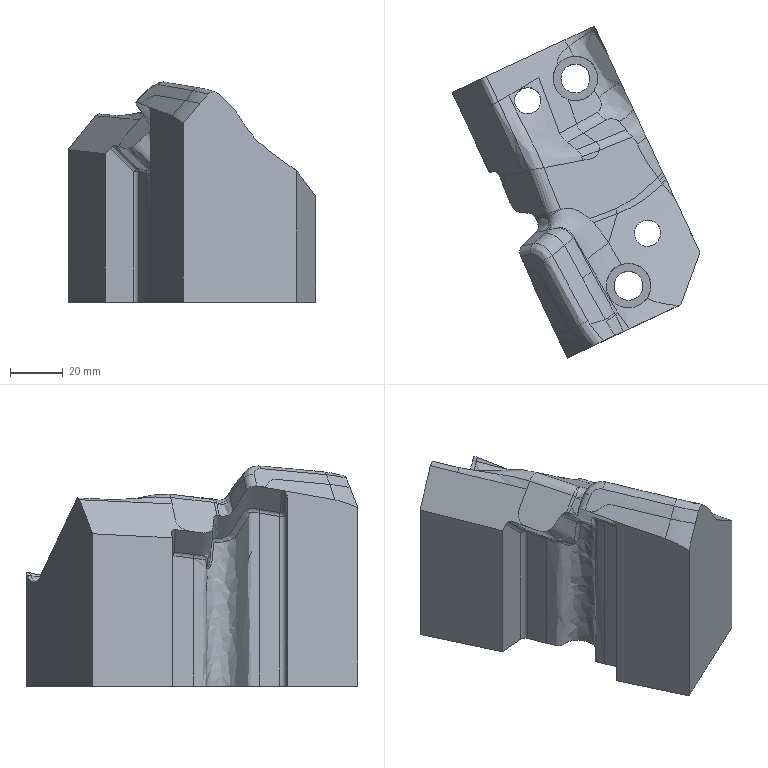Part | NX | features solid 2 | 1 solid | 91 faces | box 94.32 x 126.222 x 83.766 mm | volume 330590 mm3 | spline 70 | cylinder 10 | plane 9 | sphere 2 | commonest cylinder face diameters 4 x4 10 x2 11 x2 17 x2